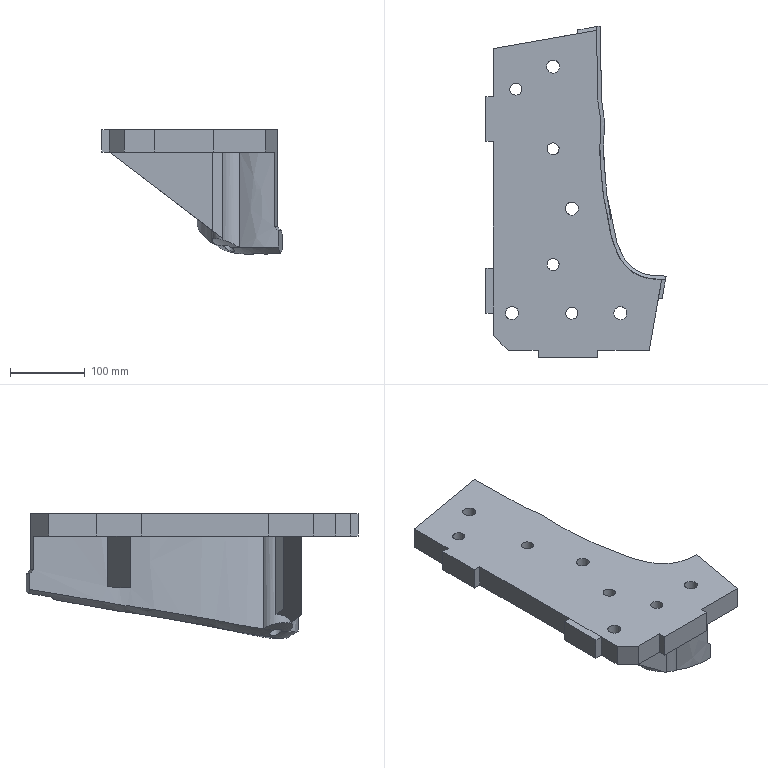Part | NX | features solid 2 | 1 solid | 69 faces | box 241.313 x 444.589 x 167.056 mm | volume 3544609 mm3 | plane 36 | cylinder 17 | spline 15 | cone 1 | commonest cylinder face diameters 16 x5 17.5 x4 25.5 x4 40 x2 14.5 x1 45 x1